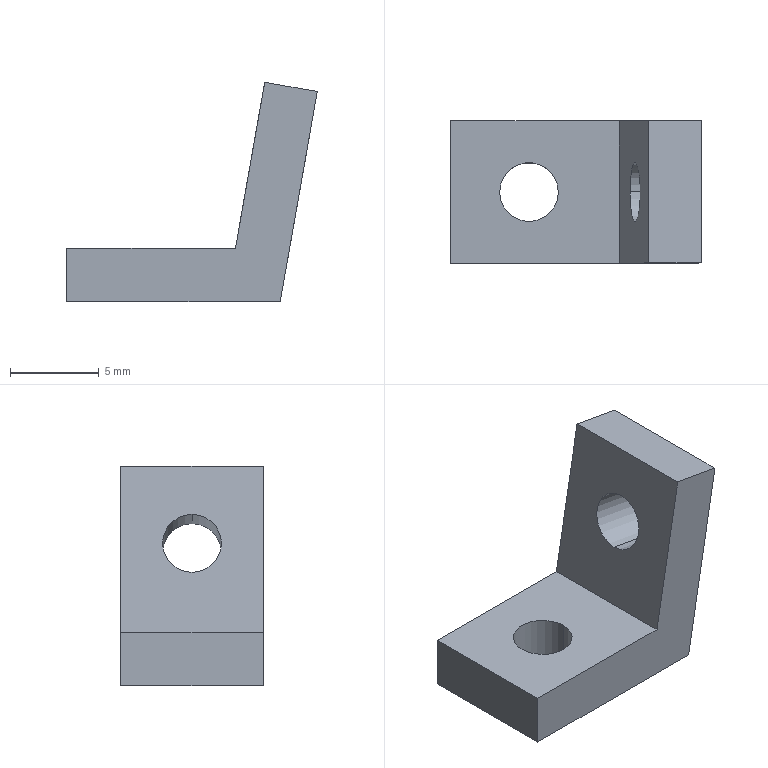Part | SolidWorks | features ICE 3, Extrusion 1 | 1 solid | 12 faces | box 14.084 x 8 x 12.339 mm | volume 464.267 mm3 | plane 8 | cylinder 4 | commonest cylinder face diameters 3.3 x4
STEP:
#1=CARTESIAN_POINT('',(3.252,0.,9.63));
#2=VERTEX_POINT('',#1);
#3=CARTESIAN_POINT('',(2.679,0.,6.381));
#4=VERTEX_POINT('',#3);
#5=CARTESIAN_POINT('',(2.965,0.,8.005));
#6=DIRECTION('',(0.9848,0.,-0.1736));
#7=DIRECTION('',(-0.1736,0.,-0.9848));
#8=AXIS2_PLACEMENT_3D('',#5,#6,#7);
#9=CIRCLE('',#8,1.65);
#10=EDGE_CURVE('',#2,#4,#9,.T.);
#11=ORIENTED_EDGE('',*,*,#10,.F.);
#12=CARTESIAN_POINT('',(6.206,0.,9.109));
#13=VERTEX_POINT('',#12);
#14=CARTESIAN_POINT('',(3.252,0.,9.63));
#15=DIRECTION('',(0.9848,0.,-0.1736));
#16=VECTOR('',#15,1000.);
#17=LINE('',#14,#16);
#18=EDGE_CURVE('',#2,#13,#17,.T.);
#19=ORIENTED_EDGE('',*,*,#18,.T.);
#20=CARTESIAN_POINT('',(5.633,0.,5.86));
#21=VERTEX_POINT('',#20);
#22=CARTESIAN_POINT('',(5.92,0.,7.485));
#23=DIRECTION('',(0.9848,0.,-0.1736));
#24=DIRECTION('',(-0.1736,0.,-0.9848));
#25=AXIS2_PLACEMENT_3D('',#22,#23,#24);
#26=CIRCLE('',#25,1.65);
#27=EDGE_CURVE('',#13,#21,#26,.T.);
#28=ORIENTED_EDGE('',*,*,#27,.T.);
#29=CARTESIAN_POINT('',(2.679,0.,6.381));
#30=DIRECTION('',(0.9848,0.,-0.1736));
#31=VECTOR('',#30,1000.);
#32=LINE('',#29,#31);
#33=EDGE_CURVE('',#4,#21,#32,.T.);
#34=ORIENTED_EDGE('',*,*,#33,.F.);
#35=EDGE_LOOP('',(#11,#19,#28,#34));
#36=FACE_OUTER_BOUND('',#35,.T.);
#37=CARTESIAN_POINT('',(2.965,0.,8.005));
#38=DIRECTION('',(0.9848,0.,-0.1736));
#39=DIRECTION('',(-0.1736,0.,-0.9848));
#40=AXIS2_PLACEMENT_3D('',#37,#38,#39);
#41=CYLINDRICAL_SURFACE('',#40,1.65);
#42=ADVANCED_FACE('',(#36),#41,.F.);
#43=CARTESIAN_POINT('',(-4.65,0.,0.));
#44=VERTEX_POINT('',#43);
#45=CARTESIAN_POINT('',(-1.35,0.,0.));
#46=VERTEX_POINT('',#45);
#47=CARTESIAN_POINT('',(-3.,0.,0.));
#48=DIRECTION('',(0.,0.,1.));
#49=DIRECTION('',(1.,0.,0.));
#50=AXIS2_PLACEMENT_3D('',#47,#48,#49);
#51=CIRCLE('',#50,1.65);
#52=EDGE_CURVE('',#44,#46,#51,.T.);
#53=ORIENTED_EDGE('',*,*,#52,.F.);
#54=CARTESIAN_POINT('',(-4.65,0.,3.));
#55=VERTEX_POINT('',#54);
#56=CARTESIAN_POINT('',(-4.65,0.,0.));
#57=DIRECTION('',(0.,0.,1.));
#58=VECTOR('',#57,1000.);
#59=LINE('',#56,#58);
#60=EDGE_CURVE('',#44,#55,#59,.T.);
#61=ORIENTED_EDGE('',*,*,#60,.T.);
#62=CARTESIAN_POINT('',(-1.35,0.,3.));
#63=VERTEX_POINT('',#62);
#64=CARTESIAN_POINT('',(-3.,0.,3.));
#65=DIRECTION('',(0.,0.,1.));
#66=DIRECTION('',(1.,0.,0.));
#67=AXIS2_PLACEMENT_3D('',#64,#65,#66);
#68=CIRCLE('',#67,1.65);
#69=EDGE_CURVE('',#55,#63,#68,.T.);
#70=ORIENTED_EDGE('',*,*,#69,.T.);
#71=CARTESIAN_POINT('',(-1.35,0.,0.));
#72=DIRECTION('',(0.,0.,1.));
#73=VECTOR('',#72,1000.);
#74=LINE('',#71,#73);
#75=EDGE_CURVE('',#46,#63,#74,.T.);
#76=ORIENTED_EDGE('',*,*,#75,.F.);
#77=EDGE_LOOP('',(#53,#61,#70,#76));
#78=FACE_OUTER_BOUND('',#77,.T.);
#79=CARTESIAN_POINT('',(-3.,0.,0.));
#80=DIRECTION('',(0.,0.,1.));
#81=DIRECTION('',(1.,0.,0.));
#82=AXIS2_PLACEMENT_3D('',#79,#80,#81);
#83=CYLINDRICAL_SURFACE('',#82,1.65);
#84=ADVANCED_FACE('',(#78),#83,.F.);
#85=CARTESIAN_POINT('',(-7.4,4.,0.));
#86=VERTEX_POINT('',#85);
#87=CARTESIAN_POINT('',(-7.4,-4.,0.));
#88=VERTEX_POINT('',#87);
#89=CARTESIAN_POINT('',(-7.4,4.,0.));
#90=DIRECTION('',(0.,-1.,0.));
#91=VECTOR('',#90,1000.);
#92=LINE('',#89,#91);
#93=EDGE_CURVE('',#86,#88,#92,.T.);
#94=ORIENTED_EDGE('',*,*,#93,.T.);
#95=CARTESIAN_POINT('',(-7.4,-4.,3.));
#96=VERTEX_POINT('',#95);
#97=CARTESIAN_POINT('',(-7.4,-4.,3.));
#98=DIRECTION('',(0.,0.,-1.));
#99=VECTOR('',#98,1000.);
#100=LINE('',#97,#99);
#101=EDGE_CURVE('',#96,#88,#100,.T.);
#102=ORIENTED_EDGE('',*,*,#101,.F.);
#103=CARTESIAN_POINT('',(-7.4,4.,3.));
#104=VERTEX_POINT('',#103);
#105=CARTESIAN_POINT('',(-7.4,4.,3.));
#106=DIRECTION('',(0.,-1.,0.));
#107=VECTOR('',#106,1000.);
#108=LINE('',#105,#107);
#109=EDGE_CURVE('',#104,#96,#108,.T.);
#110=ORIENTED_EDGE('',*,*,#109,.F.);
#111=CARTESIAN_POINT('',(-7.4,4.,3.));
#112=DIRECTION('',(0.,0.,-1.));
#113=VECTOR('',#112,1000.);
#114=LINE('',#111,#113);
#115=EDGE_CURVE('',#104,#86,#114,.T.);
#116=ORIENTED_EDGE('',*,*,#115,.T.);
#117=EDGE_LOOP('',(#94,#102,#110,#116));
#118=FACE_OUTER_BOUND('',#117,.T.);
#119=CARTESIAN_POINT('',(-7.4,4.,3.));
#120=DIRECTION('',(1.,0.,0.));
#121=DIRECTION('',(0.,0.,-1.));
#122=AXIS2_PLACEMENT_3D('',#119,#120,#121);
#123=PLANE('',#122);
#124=ADVANCED_FACE('',(#118),#123,.F.);
#125=CARTESIAN_POINT('',(4.6,-4.,0.));
#126=VERTEX_POINT('',#125);
#127=CARTESIAN_POINT('',(-7.4,-4.,0.));
#128=DIRECTION('',(1.,0.,0.));
#129=VECTOR('',#128,1000.);
#130=LINE('',#127,#129);
#131=EDGE_CURVE('',#88,#126,#130,.T.);
#132=ORIENTED_EDGE('',*,*,#131,.T.);
#133=CARTESIAN_POINT('',(6.684,-4.,11.818));
#134=VERTEX_POINT('',#133);
#135=CARTESIAN_POINT('',(4.6,-4.,0.));
#136=DIRECTION('',(0.1736,0.,0.9848));
#137=VECTOR('',#136,1000.);
#138=LINE('',#135,#137);
#139=EDGE_CURVE('',#126,#134,#138,.T.);
#140=ORIENTED_EDGE('',*,*,#139,.T.);
#141=CARTESIAN_POINT('',(3.729,-4.,12.339));
#142=VERTEX_POINT('',#141);
#143=CARTESIAN_POINT('',(6.684,-4.,11.818));
#144=DIRECTION('',(-0.9848,0.,0.1736));
#145=VECTOR('',#144,1000.);
#146=LINE('',#143,#145);
#147=EDGE_CURVE('',#134,#142,#146,.T.);
#148=ORIENTED_EDGE('',*,*,#147,.T.);
#149=CARTESIAN_POINT('',(2.083,-4.,3.));
#150=VERTEX_POINT('',#149);
#151=CARTESIAN_POINT('',(3.729,-4.,12.339));
#152=DIRECTION('',(-0.1736,0.,-0.9848));
#153=VECTOR('',#152,1000.);
#154=LINE('',#151,#153);
#155=EDGE_CURVE('',#142,#150,#154,.T.);
#156=ORIENTED_EDGE('',*,*,#155,.T.);
#157=CARTESIAN_POINT('',(-7.4,-4.,3.));
#158=DIRECTION('',(1.,0.,0.));
#159=VECTOR('',#158,1000.);
#160=LINE('',#157,#159);
#161=EDGE_CURVE('',#96,#150,#160,.T.);
#162=ORIENTED_EDGE('',*,*,#161,.F.);
#163=ORIENTED_EDGE('',*,*,#101,.T.);
#164=EDGE_LOOP('',(#132,#140,#148,#156,#162,#163));
#165=FACE_OUTER_BOUND('',#164,.T.);
#166=CARTESIAN_POINT('',(-7.4,-4.,3.));
#167=DIRECTION('',(0.,1.,0.));
#168=DIRECTION('',(0.,0.,1.));
#169=AXIS2_PLACEMENT_3D('',#166,#167,#168);
#170=PLANE('',#169);
#171=ADVANCED_FACE('',(#165),#170,.F.);
#172=CARTESIAN_POINT('',(6.684,4.,11.818));
#173=VERTEX_POINT('',#172);
#174=CARTESIAN_POINT('',(4.6,4.,0.));
#175=VERTEX_POINT('',#174);
#176=CARTESIAN_POINT('',(4.6,4.,0.));
#177=DIRECTION('',(-0.1736,0.,-0.9848));
#178=VECTOR('',#177,1000.);
#179=LINE('',#176,#178);
#180=EDGE_CURVE('',#173,#175,#179,.T.);
#181=ORIENTED_EDGE('',*,*,#180,.T.);
#182=CARTESIAN_POINT('',(-7.4,4.,0.));
#183=DIRECTION('',(-1.,0.,0.));
#184=VECTOR('',#183,1000.);
#185=LINE('',#182,#184);
#186=EDGE_CURVE('',#175,#86,#185,.T.);
#187=ORIENTED_EDGE('',*,*,#186,.T.);
#188=ORIENTED_EDGE('',*,*,#115,.F.);
#189=CARTESIAN_POINT('',(2.083,4.,3.));
#190=VERTEX_POINT('',#189);
#191=CARTESIAN_POINT('',(-7.4,4.,3.));
#192=DIRECTION('',(-1.,0.,0.));
#193=VECTOR('',#192,1000.);
#194=LINE('',#191,#193);
#195=EDGE_CURVE('',#190,#104,#194,.T.);
#196=ORIENTED_EDGE('',*,*,#195,.F.);
#197=CARTESIAN_POINT('',(3.729,4.,12.339));
#198=VERTEX_POINT('',#197);
#199=CARTESIAN_POINT('',(3.729,4.,12.339));
#200=DIRECTION('',(0.1736,0.,0.9848));
#201=VECTOR('',#200,1000.);
#202=LINE('',#199,#201);
#203=EDGE_CURVE('',#190,#198,#202,.T.);
#204=ORIENTED_EDGE('',*,*,#203,.T.);
#205=CARTESIAN_POINT('',(6.684,4.,11.818));
#206=DIRECTION('',(0.9848,0.,-0.1736));
#207=VECTOR('',#206,1000.);
#208=LINE('',#205,#207);
#209=EDGE_CURVE('',#198,#173,#208,.T.);
#210=ORIENTED_EDGE('',*,*,#209,.T.);
#211=EDGE_LOOP('',(#181,#187,#188,#196,#204,#210));
#212=FACE_OUTER_BOUND('',#211,.T.);
#213=CARTESIAN_POINT('',(-7.4,4.,3.));
#214=DIRECTION('',(0.,-1.,0.));
#215=DIRECTION('',(0.,0.,-1.));
#216=AXIS2_PLACEMENT_3D('',#213,#214,#215);
#217=PLANE('',#216);
#218=ADVANCED_FACE('',(#212),#217,.F.);
#219=CARTESIAN_POINT('',(-3.,0.,3.));
#220=DIRECTION('',(0.,0.,1.));
#221=DIRECTION('',(1.,0.,0.));
#222=AXIS2_PLACEMENT_3D('',#219,#220,#221);
#223=CIRCLE('',#222,1.65);
#224=EDGE_CURVE('',#63,#55,#223,.T.);
#225=ORIENTED_EDGE('',*,*,#224,.F.);
#226=ORIENTED_EDGE('',*,*,#69,.F.);
#227=EDGE_LOOP('',(#225,#226));
#228=FACE_BOUND('',#227,.T.);
#229=CARTESIAN_POINT('',(2.083,17.169,3.));
#230=DIRECTION('',(0.,-1.,0.));
#231=VECTOR('',#230,1000.);
#232=LINE('',#229,#231);
#233=EDGE_CURVE('',#190,#150,#232,.T.);
#234=ORIENTED_EDGE('',*,*,#233,.F.);
#235=ORIENTED_EDGE('',*,*,#195,.T.);
#236=ORIENTED_EDGE('',*,*,#109,.T.);
#237=ORIENTED_EDGE('',*,*,#161,.T.);
#238=EDGE_LOOP('',(#234,#235,#236,#237));
#239=FACE_OUTER_BOUND('',#238,.T.);
#240=CARTESIAN_POINT('',(0.,0.,3.));
#241=DIRECTION('',(0.,0.,1.));
#242=DIRECTION('',(1.,0.,0.));
#243=AXIS2_PLACEMENT_3D('',#240,#241,#242);
#244=PLANE('',#243);
#245=ADVANCED_FACE('',(#228,#239),#244,.T.);
#246=CARTESIAN_POINT('',(-3.,0.,0.));
#247=DIRECTION('',(0.,0.,1.));
#248=DIRECTION('',(1.,0.,0.));
#249=AXIS2_PLACEMENT_3D('',#246,#247,#248);
#250=CIRCLE('',#249,1.65);
#251=EDGE_CURVE('',#46,#44,#250,.T.);
#252=ORIENTED_EDGE('',*,*,#251,.T.);
#253=ORIENTED_EDGE('',*,*,#52,.T.);
#254=EDGE_LOOP('',(#252,#253));
#255=FACE_BOUND('',#254,.T.);
#256=ORIENTED_EDGE('',*,*,#93,.F.);
#257=ORIENTED_EDGE('',*,*,#186,.F.);
#258=CARTESIAN_POINT('',(4.6,4.,0.));
#259=DIRECTION('',(0.,1.,0.));
#260=VECTOR('',#259,1000.);
#261=LINE('',#258,#260);
#262=EDGE_CURVE('',#126,#175,#261,.T.);
#263=ORIENTED_EDGE('',*,*,#262,.F.);
#264=ORIENTED_EDGE('',*,*,#131,.F.);
#265=EDGE_LOOP('',(#256,#257,#263,#264));
#266=FACE_OUTER_BOUND('',#265,.T.);
#267=CARTESIAN_POINT('',(0.,0.,0.));
#268=DIRECTION('',(0.,0.,1.));
#269=DIRECTION('',(1.,0.,0.));
#270=AXIS2_PLACEMENT_3D('',#267,#268,#269);
#271=PLANE('',#270);
#272=ADVANCED_FACE('',(#255,#266),#271,.F.);
#273=CARTESIAN_POINT('',(2.965,0.,8.005));
#274=DIRECTION('',(0.9848,0.,-0.1736));
#275=DIRECTION('',(-0.1736,0.,-0.9848));
#276=AXIS2_PLACEMENT_3D('',#273,#274,#275);
#277=CIRCLE('',#276,1.65);
#278=EDGE_CURVE('',#4,#2,#277,.T.);
#279=ORIENTED_EDGE('',*,*,#278,.T.);
#280=ORIENTED_EDGE('',*,*,#10,.T.);
#281=EDGE_LOOP('',(#279,#280));
#282=FACE_BOUND('',#281,.T.);
#283=ORIENTED_EDGE('',*,*,#203,.F.);
#284=ORIENTED_EDGE('',*,*,#233,.T.);
#285=ORIENTED_EDGE('',*,*,#155,.F.);
#286=CARTESIAN_POINT('',(3.729,17.169,12.339));
#287=DIRECTION('',(0.,-1.,0.));
#288=VECTOR('',#287,1000.);
#289=LINE('',#286,#288);
#290=EDGE_CURVE('',#198,#142,#289,.T.);
#291=ORIENTED_EDGE('',*,*,#290,.F.);
#292=EDGE_LOOP('',(#283,#284,#285,#291));
#293=FACE_OUTER_BOUND('',#292,.T.);
#294=CARTESIAN_POINT('',(3.729,17.169,12.339));
#295=DIRECTION('',(-0.9848,0.,0.1736));
#296=DIRECTION('',(0.1736,0.,0.9848));
#297=AXIS2_PLACEMENT_3D('',#294,#295,#296);
#298=PLANE('',#297);
#299=ADVANCED_FACE('',(#282,#293),#298,.T.);
#300=ORIENTED_EDGE('',*,*,#209,.F.);
#301=ORIENTED_EDGE('',*,*,#290,.T.);
#302=ORIENTED_EDGE('',*,*,#147,.F.);
#303=CARTESIAN_POINT('',(6.684,17.169,11.818));
#304=DIRECTION('',(0.,-1.,0.));
#305=VECTOR('',#304,1000.);
#306=LINE('',#303,#305);
#307=EDGE_CURVE('',#173,#134,#306,.T.);
#308=ORIENTED_EDGE('',*,*,#307,.F.);
#309=EDGE_LOOP('',(#300,#301,#302,#308));
#310=FACE_OUTER_BOUND('',#309,.T.);
#311=CARTESIAN_POINT('',(6.684,17.169,11.818));
#312=DIRECTION('',(0.1736,0.,0.9848));
#313=DIRECTION('',(0.9848,0.,-0.1736));
#314=AXIS2_PLACEMENT_3D('',#311,#312,#313);
#315=PLANE('',#314);
#316=ADVANCED_FACE('',(#310),#315,.T.);
#317=CARTESIAN_POINT('',(5.92,0.,7.485));
#318=DIRECTION('',(0.9848,0.,-0.1736));
#319=DIRECTION('',(-0.1736,0.,-0.9848));
#320=AXIS2_PLACEMENT_3D('',#317,#318,#319);
#321=CIRCLE('',#320,1.65);
#322=EDGE_CURVE('',#21,#13,#321,.T.);
#323=ORIENTED_EDGE('',*,*,#322,.F.);
#324=ORIENTED_EDGE('',*,*,#27,.F.);
#325=EDGE_LOOP('',(#323,#324));
#326=FACE_BOUND('',#325,.T.);
#327=ORIENTED_EDGE('',*,*,#180,.F.);
#328=ORIENTED_EDGE('',*,*,#307,.T.);
#329=ORIENTED_EDGE('',*,*,#139,.F.);
#330=ORIENTED_EDGE('',*,*,#262,.T.);
#331=EDGE_LOOP('',(#327,#328,#329,#330));
#332=FACE_OUTER_BOUND('',#331,.T.);
#333=CARTESIAN_POINT('',(4.6,17.169,0.));
#334=DIRECTION('',(0.9848,0.,-0.1736));
#335=DIRECTION('',(-0.1736,0.,-0.9848));
#336=AXIS2_PLACEMENT_3D('',#333,#334,#335);
#337=PLANE('',#336);
#338=ADVANCED_FACE('',(#326,#332),#337,.T.);
#339=ORIENTED_EDGE('',*,*,#60,.F.);
#340=ORIENTED_EDGE('',*,*,#251,.F.);
#341=ORIENTED_EDGE('',*,*,#75,.T.);
#342=ORIENTED_EDGE('',*,*,#224,.T.);
#343=EDGE_LOOP('',(#339,#340,#341,#342));
#344=FACE_OUTER_BOUND('',#343,.T.);
#345=CARTESIAN_POINT('',(-3.,0.,0.));
#346=DIRECTION('',(0.,0.,1.));
#347=DIRECTION('',(1.,0.,0.));
#348=AXIS2_PLACEMENT_3D('',#345,#346,#347);
#349=CYLINDRICAL_SURFACE('',#348,1.65);
#350=ADVANCED_FACE('',(#344),#349,.F.);
#351=ORIENTED_EDGE('',*,*,#18,.F.);
#352=ORIENTED_EDGE('',*,*,#278,.F.);
#353=ORIENTED_EDGE('',*,*,#33,.T.);
#354=ORIENTED_EDGE('',*,*,#322,.T.);
#355=EDGE_LOOP('',(#351,#352,#353,#354));
#356=FACE_OUTER_BOUND('',#355,.T.);
#357=CARTESIAN_POINT('',(2.965,0.,8.005));
#358=DIRECTION('',(0.9848,0.,-0.1736));
#359=DIRECTION('',(-0.1736,0.,-0.9848));
#360=AXIS2_PLACEMENT_3D('',#357,#358,#359);
#361=CYLINDRICAL_SURFACE('',#360,1.65);
#362=ADVANCED_FACE('',(#356),#361,.F.);
#363=CLOSED_SHELL('',(#42,#84,#124,#171,#218,#245,#272,#299,#316,#338,#350,#362));
#364=MANIFOLD_SOLID_BREP('',#363);
#365=CARTESIAN_POINT('',(0.,0.,0.));
#366=DIRECTION('',(0.,0.,1.));
#367=DIRECTION('',(1.,0.,0.));
#368=AXIS2_PLACEMENT_3D('',#365,#366,#367);
#369=(LENGTH_UNIT()NAMED_UNIT(*)SI_UNIT(.MILLI.,.METRE.));
#370=UNCERTAINTY_MEASURE_WITH_UNIT(LENGTH_MEASURE(0.00001),#369,'','');
#371=(NAMED_UNIT(*)PLANE_ANGLE_UNIT()SI_UNIT($,.RADIAN.));
#372=(NAMED_UNIT(*)SI_UNIT($,.STERADIAN.)SOLID_ANGLE_UNIT());
#373=(GEOMETRIC_REPRESENTATION_CONTEXT(3)GLOBAL_UNCERTAINTY_ASSIGNED_CONTEXT((#370))GLOBAL_UNIT_ASSIGNED_CONTEXT((#369,#371,#372))REPRESENTATION_CONTEXT('',''));
#374=ADVANCED_BREP_SHAPE_REPRESENTATION('',(#364,#368),#373);